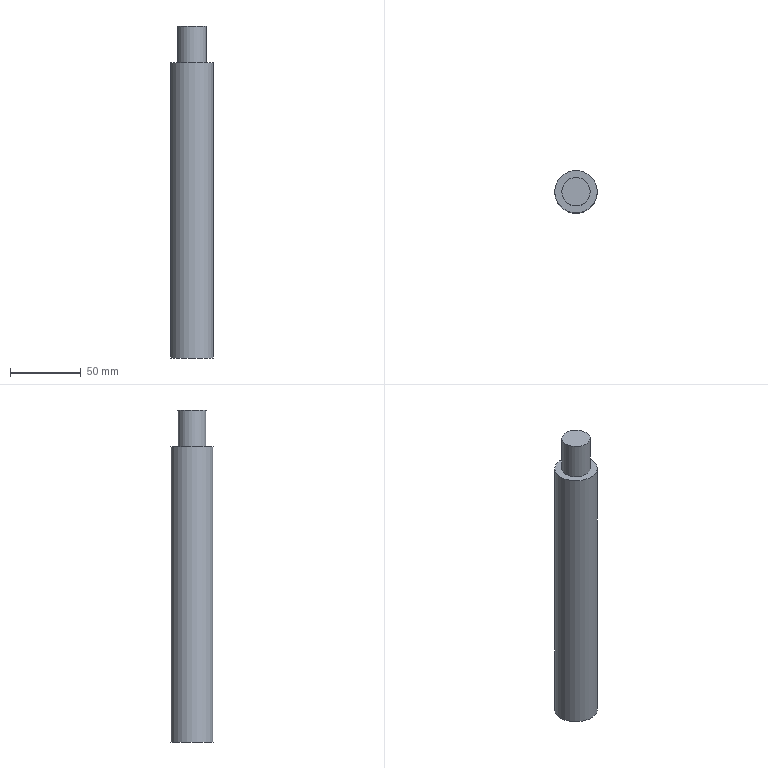Part | NX | features solid 2 | 1 solid | 5 faces | box 30 x 30 x 234 mm | volume 155195 mm3 | plane 3 | cylinder 2 | commonest cylinder face diameters 20 x1 30 x1
STEP:
#1=CARTESIAN_POINT('',(-95.,-440.,-328.));
#2=VERTEX_POINT('',#1);
#3=CARTESIAN_POINT('',(-80.,-440.,-328.));
#4=DIRECTION('',(0.,0.,1.));
#5=DIRECTION('',(-1.,0.,0.));
#6=AXIS2_PLACEMENT_3D('',#3,#4,#5);
#7=CIRCLE('',#6,15.);
#8=EDGE_CURVE('',#2,#2,#7,.T.);
#9=ORIENTED_EDGE('',*,*,#8,.T.);
#10=EDGE_LOOP('',(#9));
#11=FACE_BOUND('',#10,.T.);
#12=CARTESIAN_POINT('',(-95.,-440.,-120.));
#13=VERTEX_POINT('',#12);
#14=CARTESIAN_POINT('',(-80.,-440.,-120.));
#15=DIRECTION('',(0.,0.,1.));
#16=DIRECTION('',(-1.,0.,0.));
#17=AXIS2_PLACEMENT_3D('',#14,#15,#16);
#18=CIRCLE('',#17,15.);
#19=EDGE_CURVE('',#13,#13,#18,.T.);
#20=ORIENTED_EDGE('',*,*,#19,.F.);
#21=EDGE_LOOP('',(#20));
#22=FACE_BOUND('',#21,.T.);
#23=CARTESIAN_POINT('',(-80.,-440.,-430.));
#24=DIRECTION('',(0.,0.,1.));
#25=DIRECTION('',(-1.,0.,0.));
#26=AXIS2_PLACEMENT_3D('',#23,#24,#25);
#27=CYLINDRICAL_SURFACE('',#26,15.);
#28=ADVANCED_FACE('',(#11,#22),#27,.T.);
#29=ORIENTED_EDGE('',*,*,#8,.F.);
#30=EDGE_LOOP('',(#29));
#31=FACE_BOUND('',#30,.T.);
#32=CARTESIAN_POINT('',(-80.,-440.,-328.));
#33=DIRECTION('',(0.,0.,-1.));
#34=DIRECTION('',(1.,0.,0.));
#35=AXIS2_PLACEMENT_3D('',#32,#33,#34);
#36=PLANE('',#35);
#37=ADVANCED_FACE('',(#31),#36,.T.);
#38=CARTESIAN_POINT('',(-90.,-440.,-120.));
#39=VERTEX_POINT('',#38);
#40=CARTESIAN_POINT('',(-80.,-440.,-120.));
#41=DIRECTION('',(0.,0.,1.));
#42=DIRECTION('',(-1.,0.,0.));
#43=AXIS2_PLACEMENT_3D('',#40,#41,#42);
#44=CIRCLE('',#43,10.);
#45=EDGE_CURVE('',#39,#39,#44,.T.);
#46=ORIENTED_EDGE('',*,*,#45,.F.);
#47=EDGE_LOOP('',(#46));
#48=FACE_BOUND('',#47,.T.);
#49=ORIENTED_EDGE('',*,*,#19,.T.);
#50=EDGE_LOOP('',(#49));
#51=FACE_BOUND('',#50,.T.);
#52=CARTESIAN_POINT('',(-80.,-440.,-120.));
#53=DIRECTION('',(0.,0.,-1.));
#54=DIRECTION('',(1.,0.,0.));
#55=AXIS2_PLACEMENT_3D('',#52,#53,#54);
#56=PLANE('',#55);
#57=ADVANCED_FACE('',(#48,#51),#56,.F.);
#58=CARTESIAN_POINT('',(-70.,-440.,-94.));
#59=VERTEX_POINT('',#58);
#60=CARTESIAN_POINT('',(-80.,-440.,-94.));
#61=DIRECTION('',(0.,0.,1.));
#62=DIRECTION('',(1.,0.,0.));
#63=AXIS2_PLACEMENT_3D('',#60,#61,#62);
#64=CIRCLE('',#63,10.);
#65=EDGE_CURVE('',#59,#59,#64,.T.);
#66=ORIENTED_EDGE('',*,*,#65,.F.);
#67=EDGE_LOOP('',(#66));
#68=FACE_BOUND('',#67,.T.);
#69=ORIENTED_EDGE('',*,*,#45,.T.);
#70=EDGE_LOOP('',(#69));
#71=FACE_BOUND('',#70,.T.);
#72=CARTESIAN_POINT('',(-80.,-440.,-90.));
#73=DIRECTION('',(0.,0.,-1.));
#74=DIRECTION('',(1.,0.,0.));
#75=AXIS2_PLACEMENT_3D('',#72,#73,#74);
#76=CYLINDRICAL_SURFACE('',#75,10.);
#77=ADVANCED_FACE('',(#68,#71),#76,.T.);
#78=ORIENTED_EDGE('',*,*,#65,.T.);
#79=EDGE_LOOP('',(#78));
#80=FACE_BOUND('',#79,.T.);
#81=CARTESIAN_POINT('',(-80.,-440.,-94.));
#82=DIRECTION('',(0.,0.,-1.));
#83=DIRECTION('',(1.,0.,0.));
#84=AXIS2_PLACEMENT_3D('',#81,#82,#83);
#85=PLANE('',#84);
#86=ADVANCED_FACE('',(#80),#85,.F.);
#87=CLOSED_SHELL('',(#28,#37,#57,#77,#86));
#88=MANIFOLD_SOLID_BREP('',#87);
#89=(LENGTH_UNIT()NAMED_UNIT(*)SI_UNIT(.MILLI.,.METRE.));
#90=UNCERTAINTY_MEASURE_WITH_UNIT(LENGTH_MEASURE(0.00001),#89,'','');
#91=(NAMED_UNIT(*)PLANE_ANGLE_UNIT()SI_UNIT($,.RADIAN.));
#92=(NAMED_UNIT(*)SI_UNIT($,.STERADIAN.)SOLID_ANGLE_UNIT());
#93=(GEOMETRIC_REPRESENTATION_CONTEXT(3)GLOBAL_UNCERTAINTY_ASSIGNED_CONTEXT((#90))GLOBAL_UNIT_ASSIGNED_CONTEXT((#89,#91,#92))REPRESENTATION_CONTEXT('',''));
#94=ADVANCED_BREP_SHAPE_REPRESENTATION('',(#88),#93);